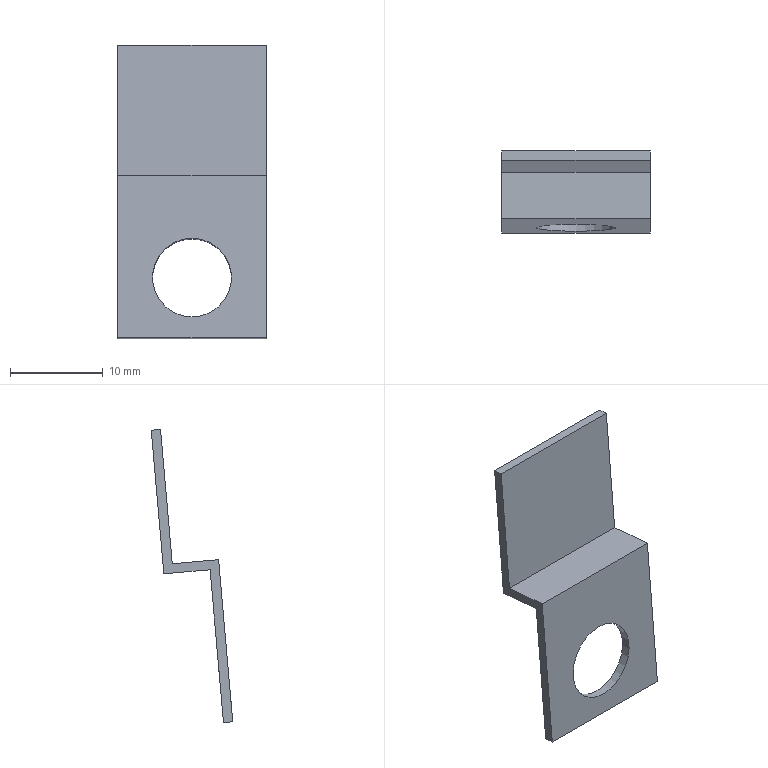Part | NX | features solid 2 | 1 solid | 11 faces | box 16 x 8.766 x 31.53 mm | volume 535.255 mm3 | plane 10 | cylinder 1 | commonest cylinder face diameters 8.5 x1
STEP:
#1=CARTESIAN_POINT('',(-128.452,-103.089,-55.618));
#2=VERTEX_POINT('',#1);
#3=CARTESIAN_POINT('',(-112.452,-103.089,-55.618));
#4=VERTEX_POINT('',#3);
#5=CARTESIAN_POINT('',(-128.452,-103.089,-55.618));
#6=DIRECTION('',(1.,0.,0.));
#7=VECTOR('',#6,1000.);
#8=LINE('',#5,#7);
#9=EDGE_CURVE('',#2,#4,#8,.T.);
#10=ORIENTED_EDGE('',*,*,#9,.F.);
#11=CARTESIAN_POINT('',(-128.452,-104.615,-73.051));
#12=VERTEX_POINT('',#11);
#13=CARTESIAN_POINT('',(-128.452,-103.177,-56.614));
#14=DIRECTION('',(0.,0.08716,0.9962));
#15=VECTOR('',#14,1000.);
#16=LINE('',#13,#15);
#17=EDGE_CURVE('',#12,#2,#16,.T.);
#18=ORIENTED_EDGE('',*,*,#17,.F.);
#19=CARTESIAN_POINT('',(-112.452,-104.615,-73.051));
#20=VERTEX_POINT('',#19);
#21=CARTESIAN_POINT('',(-128.452,-104.615,-73.051));
#22=DIRECTION('',(1.,0.,0.));
#23=VECTOR('',#22,1000.);
#24=LINE('',#21,#23);
#25=EDGE_CURVE('',#12,#20,#24,.T.);
#26=ORIENTED_EDGE('',*,*,#25,.T.);
#27=CARTESIAN_POINT('',(-112.452,-103.089,-55.618));
#28=DIRECTION('',(0.,-0.08716,-0.9962));
#29=VECTOR('',#28,1000.);
#30=LINE('',#27,#29);
#31=EDGE_CURVE('',#4,#20,#30,.T.);
#32=ORIENTED_EDGE('',*,*,#31,.F.);
#33=EDGE_LOOP('',(#10,#18,#26,#32));
#34=FACE_BOUND('',#33,.T.);
#35=CARTESIAN_POINT('',(-120.452,-104.418,-70.81));
#36=VERTEX_POINT('',#35);
#37=CARTESIAN_POINT('',(-120.452,-104.048,-66.576));
#38=DIRECTION('',(0.,0.9962,-0.08716));
#39=DIRECTION('',(0.,-0.08716,-0.9962));
#40=AXIS2_PLACEMENT_3D('',#37,#38,#39);
#41=CIRCLE('',#40,4.25);
#42=EDGE_CURVE('',#36,#36,#41,.T.);
#43=ORIENTED_EDGE('',*,*,#42,.T.);
#44=EDGE_LOOP('',(#43));
#45=FACE_BOUND('',#44,.T.);
#46=CARTESIAN_POINT('',(-112.452,-103.089,-55.618));
#47=DIRECTION('',(0.,0.9962,-0.08716));
#48=DIRECTION('',(0.,-0.08716,-0.9962));
#49=AXIS2_PLACEMENT_3D('',#46,#47,#48);
#50=PLANE('',#49);
#51=ADVANCED_FACE('',(#34,#45),#50,.F.);
#52=CARTESIAN_POINT('',(-128.452,-103.618,-73.138));
#53=VERTEX_POINT('',#52);
#54=CARTESIAN_POINT('',(-112.452,-103.618,-73.138));
#55=VERTEX_POINT('',#54);
#56=CARTESIAN_POINT('',(-128.452,-103.618,-73.138));
#57=DIRECTION('',(1.,0.,0.));
#58=VECTOR('',#57,1000.);
#59=LINE('',#56,#58);
#60=EDGE_CURVE('',#53,#55,#59,.T.);
#61=ORIENTED_EDGE('',*,*,#60,.F.);
#62=CARTESIAN_POINT('',(-128.452,-102.18,-56.701));
#63=VERTEX_POINT('',#62);
#64=CARTESIAN_POINT('',(-128.452,-102.18,-56.701));
#65=DIRECTION('',(0.,-0.08716,-0.9962));
#66=VECTOR('',#65,1000.);
#67=LINE('',#64,#66);
#68=EDGE_CURVE('',#63,#53,#67,.T.);
#69=ORIENTED_EDGE('',*,*,#68,.F.);
#70=CARTESIAN_POINT('',(-112.452,-102.18,-56.701));
#71=VERTEX_POINT('',#70);
#72=CARTESIAN_POINT('',(-128.452,-102.18,-56.701));
#73=DIRECTION('',(1.,0.,0.));
#74=VECTOR('',#73,1000.);
#75=LINE('',#72,#74);
#76=EDGE_CURVE('',#63,#71,#75,.T.);
#77=ORIENTED_EDGE('',*,*,#76,.T.);
#78=CARTESIAN_POINT('',(-112.452,-103.618,-73.138));
#79=DIRECTION('',(0.,0.08716,0.9962));
#80=VECTOR('',#79,1000.);
#81=LINE('',#78,#80);
#82=EDGE_CURVE('',#55,#71,#81,.T.);
#83=ORIENTED_EDGE('',*,*,#82,.F.);
#84=EDGE_LOOP('',(#61,#69,#77,#83));
#85=FACE_BOUND('',#84,.T.);
#86=CARTESIAN_POINT('',(-120.452,-103.422,-70.897));
#87=VERTEX_POINT('',#86);
#88=CARTESIAN_POINT('',(-120.452,-103.052,-66.663));
#89=DIRECTION('',(0.,0.9962,-0.08716));
#90=DIRECTION('',(0.,-0.08716,-0.9962));
#91=AXIS2_PLACEMENT_3D('',#88,#89,#90);
#92=CIRCLE('',#91,4.25);
#93=EDGE_CURVE('',#87,#87,#92,.T.);
#94=ORIENTED_EDGE('',*,*,#93,.F.);
#95=EDGE_LOOP('',(#94));
#96=FACE_BOUND('',#95,.T.);
#97=CARTESIAN_POINT('',(-112.452,-103.618,-73.138));
#98=DIRECTION('',(0.,-0.9962,0.08716));
#99=DIRECTION('',(0.,0.08716,0.9962));
#100=AXIS2_PLACEMENT_3D('',#97,#98,#99);
#101=PLANE('',#100);
#102=ADVANCED_FACE('',(#85,#96),#101,.F.);
#103=CARTESIAN_POINT('',(-112.452,-96.845,-41.609));
#104=VERTEX_POINT('',#103);
#105=CARTESIAN_POINT('',(-128.452,-96.845,-41.609));
#106=VERTEX_POINT('',#105);
#107=CARTESIAN_POINT('',(-112.452,-96.845,-41.609));
#108=DIRECTION('',(-1.,0.,0.));
#109=VECTOR('',#108,1000.);
#110=LINE('',#107,#109);
#111=EDGE_CURVE('',#104,#106,#110,.T.);
#112=ORIENTED_EDGE('',*,*,#111,.F.);
#113=CARTESIAN_POINT('',(-112.452,-95.848,-41.696));
#114=VERTEX_POINT('',#113);
#115=CARTESIAN_POINT('',(-112.452,-95.848,-41.696));
#116=DIRECTION('',(0.,-0.9962,0.08716));
#117=VECTOR('',#116,1000.);
#118=LINE('',#115,#117);
#119=EDGE_CURVE('',#114,#104,#118,.T.);
#120=ORIENTED_EDGE('',*,*,#119,.F.);
#121=CARTESIAN_POINT('',(-128.452,-95.848,-41.696));
#122=VERTEX_POINT('',#121);
#123=CARTESIAN_POINT('',(-112.452,-95.848,-41.696));
#124=DIRECTION('',(-1.,0.,0.));
#125=VECTOR('',#124,1000.);
#126=LINE('',#123,#125);
#127=EDGE_CURVE('',#114,#122,#126,.T.);
#128=ORIENTED_EDGE('',*,*,#127,.T.);
#129=CARTESIAN_POINT('',(-128.452,-95.848,-41.696));
#130=DIRECTION('',(0.,-0.9962,0.08716));
#131=VECTOR('',#130,1000.);
#132=LINE('',#129,#131);
#133=EDGE_CURVE('',#122,#106,#132,.T.);
#134=ORIENTED_EDGE('',*,*,#133,.T.);
#135=EDGE_LOOP('',(#112,#120,#128,#134));
#136=FACE_BOUND('',#135,.T.);
#137=CARTESIAN_POINT('',(-112.452,-95.848,-41.696));
#138=DIRECTION('',(0.,0.08716,0.9962));
#139=DIRECTION('',(0.,0.9962,-0.08716));
#140=AXIS2_PLACEMENT_3D('',#137,#138,#139);
#141=PLANE('',#140);
#142=ADVANCED_FACE('',(#136),#141,.T.);
#143=CARTESIAN_POINT('',(-128.452,-98.108,-56.054));
#144=VERTEX_POINT('',#143);
#145=CARTESIAN_POINT('',(-128.452,-96.845,-41.609));
#146=DIRECTION('',(0.,-0.08716,-0.9962));
#147=VECTOR('',#146,1000.);
#148=LINE('',#145,#147);
#149=EDGE_CURVE('',#106,#144,#148,.T.);
#150=ORIENTED_EDGE('',*,*,#149,.F.);
#151=ORIENTED_EDGE('',*,*,#133,.F.);
#152=CARTESIAN_POINT('',(-128.452,-97.199,-57.137));
#153=VERTEX_POINT('',#152);
#154=CARTESIAN_POINT('',(-128.452,-95.848,-41.696));
#155=DIRECTION('',(0.,-0.08716,-0.9962));
#156=VECTOR('',#155,1000.);
#157=LINE('',#154,#156);
#158=EDGE_CURVE('',#122,#153,#157,.T.);
#159=ORIENTED_EDGE('',*,*,#158,.T.);
#160=CARTESIAN_POINT('',(-128.452,-97.199,-57.137));
#161=DIRECTION('',(0.,-0.9962,0.08716));
#162=VECTOR('',#161,1000.);
#163=LINE('',#160,#162);
#164=EDGE_CURVE('',#153,#63,#163,.T.);
#165=ORIENTED_EDGE('',*,*,#164,.T.);
#166=ORIENTED_EDGE('',*,*,#68,.T.);
#167=CARTESIAN_POINT('',(-128.452,-103.618,-73.138));
#168=DIRECTION('',(0.,-0.9962,0.08716));
#169=VECTOR('',#168,1000.);
#170=LINE('',#167,#169);
#171=EDGE_CURVE('',#53,#12,#170,.T.);
#172=ORIENTED_EDGE('',*,*,#171,.T.);
#173=ORIENTED_EDGE('',*,*,#17,.T.);
#174=CARTESIAN_POINT('',(-128.452,-97.112,-56.141));
#175=DIRECTION('',(0.,-0.9962,0.08716));
#176=VECTOR('',#175,1000.);
#177=LINE('',#174,#176);
#178=EDGE_CURVE('',#144,#2,#177,.T.);
#179=ORIENTED_EDGE('',*,*,#178,.F.);
#180=EDGE_LOOP('',(#150,#151,#159,#165,#166,#172,#173,#179));
#181=FACE_BOUND('',#180,.T.);
#182=CARTESIAN_POINT('',(-128.452,-95.848,-41.696));
#183=DIRECTION('',(-1.,0.,0.));
#184=DIRECTION('',(0.,0.9962,-0.08716));
#185=AXIS2_PLACEMENT_3D('',#182,#183,#184);
#186=PLANE('',#185);
#187=ADVANCED_FACE('',(#181),#186,.T.);
#188=CARTESIAN_POINT('',(-112.452,-98.108,-56.054));
#189=VERTEX_POINT('',#188);
#190=CARTESIAN_POINT('',(-112.452,-98.108,-56.054));
#191=DIRECTION('',(0.,0.08716,0.9962));
#192=VECTOR('',#191,1000.);
#193=LINE('',#190,#192);
#194=EDGE_CURVE('',#189,#104,#193,.T.);
#195=ORIENTED_EDGE('',*,*,#194,.F.);
#196=CARTESIAN_POINT('',(-112.452,-97.112,-56.141));
#197=DIRECTION('',(0.,-0.9962,0.08716));
#198=VECTOR('',#197,1000.);
#199=LINE('',#196,#198);
#200=EDGE_CURVE('',#189,#4,#199,.T.);
#201=ORIENTED_EDGE('',*,*,#200,.T.);
#202=ORIENTED_EDGE('',*,*,#31,.T.);
#203=CARTESIAN_POINT('',(-112.452,-103.618,-73.138));
#204=DIRECTION('',(0.,-0.9962,0.08716));
#205=VECTOR('',#204,1000.);
#206=LINE('',#203,#205);
#207=EDGE_CURVE('',#55,#20,#206,.T.);
#208=ORIENTED_EDGE('',*,*,#207,.F.);
#209=ORIENTED_EDGE('',*,*,#82,.T.);
#210=CARTESIAN_POINT('',(-112.452,-97.199,-57.137));
#211=VERTEX_POINT('',#210);
#212=CARTESIAN_POINT('',(-112.452,-97.199,-57.137));
#213=DIRECTION('',(0.,-0.9962,0.08716));
#214=VECTOR('',#213,1000.);
#215=LINE('',#212,#214);
#216=EDGE_CURVE('',#211,#71,#215,.T.);
#217=ORIENTED_EDGE('',*,*,#216,.F.);
#218=CARTESIAN_POINT('',(-112.452,-97.112,-56.141));
#219=DIRECTION('',(0.,0.08716,0.9962));
#220=VECTOR('',#219,1000.);
#221=LINE('',#218,#220);
#222=EDGE_CURVE('',#211,#114,#221,.T.);
#223=ORIENTED_EDGE('',*,*,#222,.T.);
#224=ORIENTED_EDGE('',*,*,#119,.T.);
#225=EDGE_LOOP('',(#195,#201,#202,#208,#209,#217,#223,#224));
#226=FACE_BOUND('',#225,.T.);
#227=CARTESIAN_POINT('',(-112.452,-97.112,-56.141));
#228=DIRECTION('',(1.,0.,0.));
#229=DIRECTION('',(0.,-0.08716,-0.9962));
#230=AXIS2_PLACEMENT_3D('',#227,#228,#229);
#231=PLANE('',#230);
#232=ADVANCED_FACE('',(#226),#231,.T.);
#233=ORIENTED_EDGE('',*,*,#127,.F.);
#234=ORIENTED_EDGE('',*,*,#222,.F.);
#235=CARTESIAN_POINT('',(-128.452,-97.199,-57.137));
#236=DIRECTION('',(1.,0.,0.));
#237=VECTOR('',#236,1000.);
#238=LINE('',#235,#237);
#239=EDGE_CURVE('',#153,#211,#238,.T.);
#240=ORIENTED_EDGE('',*,*,#239,.F.);
#241=ORIENTED_EDGE('',*,*,#158,.F.);
#242=EDGE_LOOP('',(#233,#234,#240,#241));
#243=FACE_BOUND('',#242,.T.);
#244=CARTESIAN_POINT('',(-128.452,-95.848,-41.696));
#245=DIRECTION('',(0.,-0.9962,0.08716));
#246=DIRECTION('',(0.,0.08716,0.9962));
#247=AXIS2_PLACEMENT_3D('',#244,#245,#246);
#248=PLANE('',#247);
#249=ADVANCED_FACE('',(#243),#248,.F.);
#250=ORIENTED_EDGE('',*,*,#111,.T.);
#251=ORIENTED_EDGE('',*,*,#149,.T.);
#252=CARTESIAN_POINT('',(-128.452,-98.108,-56.054));
#253=DIRECTION('',(1.,0.,0.));
#254=VECTOR('',#253,1000.);
#255=LINE('',#252,#254);
#256=EDGE_CURVE('',#144,#189,#255,.T.);
#257=ORIENTED_EDGE('',*,*,#256,.T.);
#258=ORIENTED_EDGE('',*,*,#194,.T.);
#259=EDGE_LOOP('',(#250,#251,#257,#258));
#260=FACE_BOUND('',#259,.T.);
#261=CARTESIAN_POINT('',(-128.452,-96.845,-41.609));
#262=DIRECTION('',(0.,-0.9962,0.08716));
#263=DIRECTION('',(0.,0.08716,0.9962));
#264=AXIS2_PLACEMENT_3D('',#261,#262,#263);
#265=PLANE('',#264);
#266=ADVANCED_FACE('',(#260),#265,.T.);
#267=ORIENTED_EDGE('',*,*,#256,.F.);
#268=ORIENTED_EDGE('',*,*,#178,.T.);
#269=ORIENTED_EDGE('',*,*,#9,.T.);
#270=ORIENTED_EDGE('',*,*,#200,.F.);
#271=EDGE_LOOP('',(#267,#268,#269,#270));
#272=FACE_BOUND('',#271,.T.);
#273=CARTESIAN_POINT('',(-128.452,-97.112,-56.141));
#274=DIRECTION('',(0.,-0.08716,-0.9962));
#275=DIRECTION('',(0.,-0.9962,0.08716));
#276=AXIS2_PLACEMENT_3D('',#273,#274,#275);
#277=PLANE('',#276);
#278=ADVANCED_FACE('',(#272),#277,.F.);
#279=ORIENTED_EDGE('',*,*,#76,.F.);
#280=ORIENTED_EDGE('',*,*,#164,.F.);
#281=ORIENTED_EDGE('',*,*,#239,.T.);
#282=ORIENTED_EDGE('',*,*,#216,.T.);
#283=EDGE_LOOP('',(#279,#280,#281,#282));
#284=FACE_BOUND('',#283,.T.);
#285=CARTESIAN_POINT('',(-128.452,-97.199,-57.137));
#286=DIRECTION('',(0.,-0.08716,-0.9962));
#287=DIRECTION('',(0.,-0.9962,0.08716));
#288=AXIS2_PLACEMENT_3D('',#285,#286,#287);
#289=PLANE('',#288);
#290=ADVANCED_FACE('',(#284),#289,.T.);
#291=ORIENTED_EDGE('',*,*,#25,.F.);
#292=ORIENTED_EDGE('',*,*,#171,.F.);
#293=ORIENTED_EDGE('',*,*,#60,.T.);
#294=ORIENTED_EDGE('',*,*,#207,.T.);
#295=EDGE_LOOP('',(#291,#292,#293,#294));
#296=FACE_BOUND('',#295,.T.);
#297=CARTESIAN_POINT('',(-128.452,-103.618,-73.138));
#298=DIRECTION('',(0.,-0.08716,-0.9962));
#299=DIRECTION('',(0.,-0.9962,0.08716));
#300=AXIS2_PLACEMENT_3D('',#297,#298,#299);
#301=PLANE('',#300);
#302=ADVANCED_FACE('',(#296),#301,.T.);
#303=ORIENTED_EDGE('',*,*,#93,.T.);
#304=EDGE_LOOP('',(#303));
#305=FACE_BOUND('',#304,.T.);
#306=ORIENTED_EDGE('',*,*,#42,.F.);
#307=EDGE_LOOP('',(#306));
#308=FACE_BOUND('',#307,.T.);
#309=CARTESIAN_POINT('',(-120.452,-103.052,-66.663));
#310=DIRECTION('',(0.,-0.9962,0.08716));
#311=DIRECTION('',(0.,0.08716,0.9962));
#312=AXIS2_PLACEMENT_3D('',#309,#310,#311);
#313=CYLINDRICAL_SURFACE('',#312,4.25);
#314=ADVANCED_FACE('',(#305,#308),#313,.F.);
#315=CLOSED_SHELL('',(#51,#102,#142,#187,#232,#249,#266,#278,#290,#302,#314));
#316=MANIFOLD_SOLID_BREP('',#315);
#317=(LENGTH_UNIT()NAMED_UNIT(*)SI_UNIT(.MILLI.,.METRE.));
#318=UNCERTAINTY_MEASURE_WITH_UNIT(LENGTH_MEASURE(0.00001),#317,'','');
#319=(NAMED_UNIT(*)PLANE_ANGLE_UNIT()SI_UNIT($,.RADIAN.));
#320=(NAMED_UNIT(*)SI_UNIT($,.STERADIAN.)SOLID_ANGLE_UNIT());
#321=(GEOMETRIC_REPRESENTATION_CONTEXT(3)GLOBAL_UNCERTAINTY_ASSIGNED_CONTEXT((#318))GLOBAL_UNIT_ASSIGNED_CONTEXT((#317,#319,#320))REPRESENTATION_CONTEXT('',''));
#322=ADVANCED_BREP_SHAPE_REPRESENTATION('',(#316),#321);